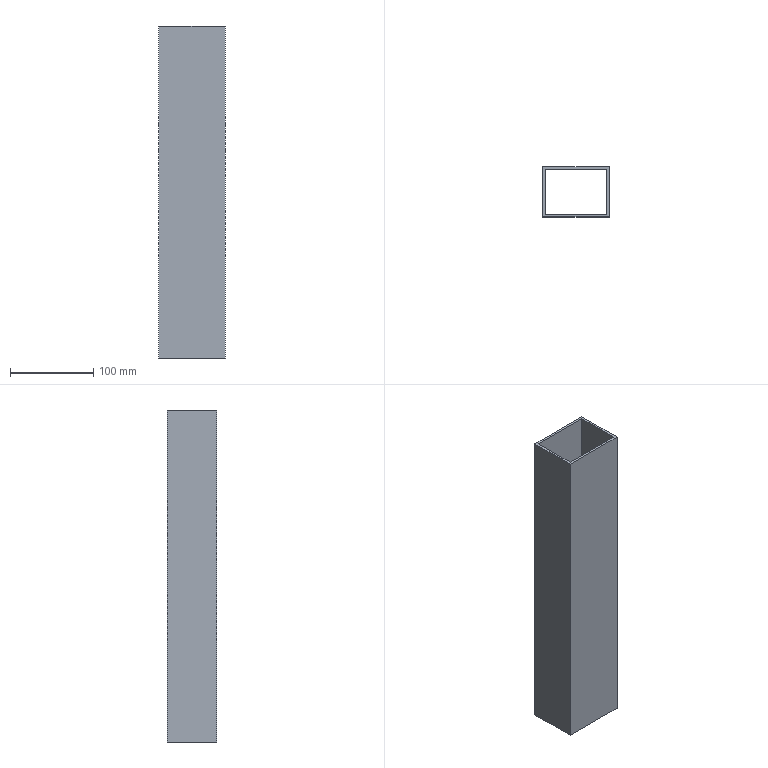Part | STEP file | Guide wheel mechanism revised.sldasm-Part-151 | 1 solid | 10 faces | box 80 x 60 x 400 mm | volume 321600 mm3 | plane 10
STEP:
#1=CARTESIAN_POINT('',(-360.,1970.,200.));
#2=VERTEX_POINT('',#1);
#3=CARTESIAN_POINT('',(-440.,1970.,200.));
#4=VERTEX_POINT('',#3);
#5=CARTESIAN_POINT('',(-440.,1970.,200.));
#6=DIRECTION('',(-1.,0.,0.));
#7=VECTOR('',#6,1000.);
#8=LINE('',#5,#7);
#9=EDGE_CURVE('',#2,#4,#8,.T.);
#10=ORIENTED_EDGE('',*,*,#9,.F.);
#11=CARTESIAN_POINT('',(-360.,1970.,-200.));
#12=VERTEX_POINT('',#11);
#13=CARTESIAN_POINT('',(-360.,1970.,300.));
#14=DIRECTION('',(0.,0.,-1.));
#15=VECTOR('',#14,1000.);
#16=LINE('',#13,#15);
#17=EDGE_CURVE('',#2,#12,#16,.T.);
#18=ORIENTED_EDGE('',*,*,#17,.T.);
#19=CARTESIAN_POINT('',(-440.,1970.,-200.));
#20=VERTEX_POINT('',#19);
#21=CARTESIAN_POINT('',(-440.,1970.,-200.));
#22=DIRECTION('',(-1.,0.,0.));
#23=VECTOR('',#22,1000.);
#24=LINE('',#21,#23);
#25=EDGE_CURVE('',#12,#20,#24,.T.);
#26=ORIENTED_EDGE('',*,*,#25,.T.);
#27=CARTESIAN_POINT('',(-440.,1970.,300.));
#28=DIRECTION('',(0.,0.,-1.));
#29=VECTOR('',#28,1000.);
#30=LINE('',#27,#29);
#31=EDGE_CURVE('',#4,#20,#30,.T.);
#32=ORIENTED_EDGE('',*,*,#31,.F.);
#33=EDGE_LOOP('',(#10,#18,#26,#32));
#34=FACE_OUTER_BOUND('',#33,.T.);
#35=CARTESIAN_POINT('',(-440.,1970.,300.));
#36=DIRECTION('',(0.,-1.,0.));
#37=DIRECTION('',(1.,0.,0.));
#38=AXIS2_PLACEMENT_3D('',#35,#36,#37);
#39=PLANE('',#38);
#40=ADVANCED_FACE('',(#34),#39,.F.);
#41=CARTESIAN_POINT('',(-360.,1910.,200.));
#42=VERTEX_POINT('',#41);
#43=CARTESIAN_POINT('',(-360.,1970.,200.));
#44=DIRECTION('',(0.,1.,0.));
#45=VECTOR('',#44,1000.);
#46=LINE('',#43,#45);
#47=EDGE_CURVE('',#42,#2,#46,.T.);
#48=ORIENTED_EDGE('',*,*,#47,.F.);
#49=CARTESIAN_POINT('',(-360.,1910.,-200.));
#50=VERTEX_POINT('',#49);
#51=CARTESIAN_POINT('',(-360.,1910.,300.));
#52=DIRECTION('',(0.,0.,-1.));
#53=VECTOR('',#52,1000.);
#54=LINE('',#51,#53);
#55=EDGE_CURVE('',#42,#50,#54,.T.);
#56=ORIENTED_EDGE('',*,*,#55,.T.);
#57=CARTESIAN_POINT('',(-360.,1970.,-200.));
#58=DIRECTION('',(0.,1.,0.));
#59=VECTOR('',#58,1000.);
#60=LINE('',#57,#59);
#61=EDGE_CURVE('',#50,#12,#60,.T.);
#62=ORIENTED_EDGE('',*,*,#61,.T.);
#63=ORIENTED_EDGE('',*,*,#17,.F.);
#64=EDGE_LOOP('',(#48,#56,#62,#63));
#65=FACE_OUTER_BOUND('',#64,.T.);
#66=CARTESIAN_POINT('',(-360.,1970.,300.));
#67=DIRECTION('',(-1.,0.,0.));
#68=DIRECTION('',(0.,0.,1.));
#69=AXIS2_PLACEMENT_3D('',#66,#67,#68);
#70=PLANE('',#69);
#71=ADVANCED_FACE('',(#65),#70,.F.);
#72=CARTESIAN_POINT('',(-440.,1910.,200.));
#73=VERTEX_POINT('',#72);
#74=CARTESIAN_POINT('',(-440.,1910.,200.));
#75=DIRECTION('',(1.,0.,0.));
#76=VECTOR('',#75,1000.);
#77=LINE('',#74,#76);
#78=EDGE_CURVE('',#73,#42,#77,.T.);
#79=ORIENTED_EDGE('',*,*,#78,.F.);
#80=CARTESIAN_POINT('',(-440.,1910.,-200.));
#81=VERTEX_POINT('',#80);
#82=CARTESIAN_POINT('',(-440.,1910.,300.));
#83=DIRECTION('',(0.,0.,-1.));
#84=VECTOR('',#83,1000.);
#85=LINE('',#82,#84);
#86=EDGE_CURVE('',#73,#81,#85,.T.);
#87=ORIENTED_EDGE('',*,*,#86,.T.);
#88=CARTESIAN_POINT('',(-440.,1910.,-200.));
#89=DIRECTION('',(1.,0.,0.));
#90=VECTOR('',#89,1000.);
#91=LINE('',#88,#90);
#92=EDGE_CURVE('',#81,#50,#91,.T.);
#93=ORIENTED_EDGE('',*,*,#92,.T.);
#94=ORIENTED_EDGE('',*,*,#55,.F.);
#95=EDGE_LOOP('',(#79,#87,#93,#94));
#96=FACE_OUTER_BOUND('',#95,.T.);
#97=CARTESIAN_POINT('',(-440.,1910.,300.));
#98=DIRECTION('',(0.,1.,0.));
#99=DIRECTION('',(0.,0.,1.));
#100=AXIS2_PLACEMENT_3D('',#97,#98,#99);
#101=PLANE('',#100);
#102=ADVANCED_FACE('',(#96),#101,.F.);
#103=CARTESIAN_POINT('',(-440.,1970.,200.));
#104=DIRECTION('',(0.,-1.,0.));
#105=VECTOR('',#104,1000.);
#106=LINE('',#103,#105);
#107=EDGE_CURVE('',#4,#73,#106,.T.);
#108=ORIENTED_EDGE('',*,*,#107,.F.);
#109=ORIENTED_EDGE('',*,*,#31,.T.);
#110=CARTESIAN_POINT('',(-440.,1970.,-200.));
#111=DIRECTION('',(0.,-1.,0.));
#112=VECTOR('',#111,1000.);
#113=LINE('',#110,#112);
#114=EDGE_CURVE('',#20,#81,#113,.T.);
#115=ORIENTED_EDGE('',*,*,#114,.T.);
#116=ORIENTED_EDGE('',*,*,#86,.F.);
#117=EDGE_LOOP('',(#108,#109,#115,#116));
#118=FACE_OUTER_BOUND('',#117,.T.);
#119=CARTESIAN_POINT('',(-440.,1970.,300.));
#120=DIRECTION('',(1.,0.,0.));
#121=DIRECTION('',(0.,0.,-1.));
#122=AXIS2_PLACEMENT_3D('',#119,#120,#121);
#123=PLANE('',#122);
#124=ADVANCED_FACE('',(#118),#123,.F.);
#125=ORIENTED_EDGE('',*,*,#114,.F.);
#126=ORIENTED_EDGE('',*,*,#25,.F.);
#127=ORIENTED_EDGE('',*,*,#61,.F.);
#128=ORIENTED_EDGE('',*,*,#92,.F.);
#129=EDGE_LOOP('',(#125,#126,#127,#128));
#130=FACE_OUTER_BOUND('',#129,.T.);
#131=CARTESIAN_POINT('',(-437.,1967.,-200.));
#132=VERTEX_POINT('',#131);
#133=CARTESIAN_POINT('',(-437.,1913.,-200.));
#134=VERTEX_POINT('',#133);
#135=CARTESIAN_POINT('',(-437.,1967.,-200.));
#136=DIRECTION('',(0.,-1.,0.));
#137=VECTOR('',#136,1000.);
#138=LINE('',#135,#137);
#139=EDGE_CURVE('',#132,#134,#138,.T.);
#140=ORIENTED_EDGE('',*,*,#139,.T.);
#141=CARTESIAN_POINT('',(-363.,1913.,-200.));
#142=VERTEX_POINT('',#141);
#143=CARTESIAN_POINT('',(-437.,1913.,-200.));
#144=DIRECTION('',(1.,0.,0.));
#145=VECTOR('',#144,1000.);
#146=LINE('',#143,#145);
#147=EDGE_CURVE('',#134,#142,#146,.T.);
#148=ORIENTED_EDGE('',*,*,#147,.T.);
#149=CARTESIAN_POINT('',(-363.,1967.,-200.));
#150=VERTEX_POINT('',#149);
#151=CARTESIAN_POINT('',(-363.,1967.,-200.));
#152=DIRECTION('',(0.,1.,0.));
#153=VECTOR('',#152,1000.);
#154=LINE('',#151,#153);
#155=EDGE_CURVE('',#142,#150,#154,.T.);
#156=ORIENTED_EDGE('',*,*,#155,.T.);
#157=CARTESIAN_POINT('',(-437.,1967.,-200.));
#158=DIRECTION('',(-1.,0.,0.));
#159=VECTOR('',#158,1000.);
#160=LINE('',#157,#159);
#161=EDGE_CURVE('',#150,#132,#160,.T.);
#162=ORIENTED_EDGE('',*,*,#161,.T.);
#163=EDGE_LOOP('',(#140,#148,#156,#162));
#164=FACE_BOUND('',#163,.T.);
#165=CARTESIAN_POINT('',(0.,0.,-200.));
#166=DIRECTION('',(0.,0.,1.));
#167=DIRECTION('',(1.,0.,0.));
#168=AXIS2_PLACEMENT_3D('',#165,#166,#167);
#169=PLANE('',#168);
#170=ADVANCED_FACE('',(#130,#164),#169,.F.);
#171=CARTESIAN_POINT('',(-363.,1967.,200.));
#172=VERTEX_POINT('',#171);
#173=CARTESIAN_POINT('',(-363.,1967.,300.));
#174=DIRECTION('',(0.,0.,-1.));
#175=VECTOR('',#174,1000.);
#176=LINE('',#173,#175);
#177=EDGE_CURVE('',#172,#150,#176,.T.);
#178=ORIENTED_EDGE('',*,*,#177,.F.);
#179=CARTESIAN_POINT('',(-437.,1967.,200.));
#180=VERTEX_POINT('',#179);
#181=CARTESIAN_POINT('',(-437.,1967.,200.));
#182=DIRECTION('',(-1.,0.,0.));
#183=VECTOR('',#182,1000.);
#184=LINE('',#181,#183);
#185=EDGE_CURVE('',#172,#180,#184,.T.);
#186=ORIENTED_EDGE('',*,*,#185,.T.);
#187=CARTESIAN_POINT('',(-437.,1967.,300.));
#188=DIRECTION('',(0.,0.,-1.));
#189=VECTOR('',#188,1000.);
#190=LINE('',#187,#189);
#191=EDGE_CURVE('',#180,#132,#190,.T.);
#192=ORIENTED_EDGE('',*,*,#191,.T.);
#193=ORIENTED_EDGE('',*,*,#161,.F.);
#194=EDGE_LOOP('',(#178,#186,#192,#193));
#195=FACE_OUTER_BOUND('',#194,.T.);
#196=CARTESIAN_POINT('',(-437.,1967.,300.));
#197=DIRECTION('',(0.,-1.,0.));
#198=DIRECTION('',(0.,0.,-1.));
#199=AXIS2_PLACEMENT_3D('',#196,#197,#198);
#200=PLANE('',#199);
#201=ADVANCED_FACE('',(#195),#200,.T.);
#202=CARTESIAN_POINT('',(-363.,1913.,200.));
#203=VERTEX_POINT('',#202);
#204=CARTESIAN_POINT('',(-363.,1913.,300.));
#205=DIRECTION('',(0.,0.,-1.));
#206=VECTOR('',#205,1000.);
#207=LINE('',#204,#206);
#208=EDGE_CURVE('',#203,#142,#207,.T.);
#209=ORIENTED_EDGE('',*,*,#208,.F.);
#210=CARTESIAN_POINT('',(-363.,1967.,200.));
#211=DIRECTION('',(0.,1.,0.));
#212=VECTOR('',#211,1000.);
#213=LINE('',#210,#212);
#214=EDGE_CURVE('',#203,#172,#213,.T.);
#215=ORIENTED_EDGE('',*,*,#214,.T.);
#216=ORIENTED_EDGE('',*,*,#177,.T.);
#217=ORIENTED_EDGE('',*,*,#155,.F.);
#218=EDGE_LOOP('',(#209,#215,#216,#217));
#219=FACE_OUTER_BOUND('',#218,.T.);
#220=CARTESIAN_POINT('',(-363.,1967.,300.));
#221=DIRECTION('',(-1.,0.,0.));
#222=DIRECTION('',(0.,0.,1.));
#223=AXIS2_PLACEMENT_3D('',#220,#221,#222);
#224=PLANE('',#223);
#225=ADVANCED_FACE('',(#219),#224,.T.);
#226=CARTESIAN_POINT('',(-437.,1913.,200.));
#227=VERTEX_POINT('',#226);
#228=CARTESIAN_POINT('',(-437.,1913.,300.));
#229=DIRECTION('',(0.,0.,-1.));
#230=VECTOR('',#229,1000.);
#231=LINE('',#228,#230);
#232=EDGE_CURVE('',#227,#134,#231,.T.);
#233=ORIENTED_EDGE('',*,*,#232,.F.);
#234=CARTESIAN_POINT('',(-437.,1913.,200.));
#235=DIRECTION('',(1.,0.,0.));
#236=VECTOR('',#235,1000.);
#237=LINE('',#234,#236);
#238=EDGE_CURVE('',#227,#203,#237,.T.);
#239=ORIENTED_EDGE('',*,*,#238,.T.);
#240=ORIENTED_EDGE('',*,*,#208,.T.);
#241=ORIENTED_EDGE('',*,*,#147,.F.);
#242=EDGE_LOOP('',(#233,#239,#240,#241));
#243=FACE_OUTER_BOUND('',#242,.T.);
#244=CARTESIAN_POINT('',(-437.,1913.,300.));
#245=DIRECTION('',(0.,1.,0.));
#246=DIRECTION('',(0.,0.,1.));
#247=AXIS2_PLACEMENT_3D('',#244,#245,#246);
#248=PLANE('',#247);
#249=ADVANCED_FACE('',(#243),#248,.T.);
#250=ORIENTED_EDGE('',*,*,#191,.F.);
#251=CARTESIAN_POINT('',(-437.,1967.,200.));
#252=DIRECTION('',(0.,-1.,0.));
#253=VECTOR('',#252,1000.);
#254=LINE('',#251,#253);
#255=EDGE_CURVE('',#180,#227,#254,.T.);
#256=ORIENTED_EDGE('',*,*,#255,.T.);
#257=ORIENTED_EDGE('',*,*,#232,.T.);
#258=ORIENTED_EDGE('',*,*,#139,.F.);
#259=EDGE_LOOP('',(#250,#256,#257,#258));
#260=FACE_OUTER_BOUND('',#259,.T.);
#261=CARTESIAN_POINT('',(-437.,1967.,300.));
#262=DIRECTION('',(1.,0.,0.));
#263=DIRECTION('',(0.,1.,0.));
#264=AXIS2_PLACEMENT_3D('',#261,#262,#263);
#265=PLANE('',#264);
#266=ADVANCED_FACE('',(#260),#265,.T.);
#267=ORIENTED_EDGE('',*,*,#255,.F.);
#268=ORIENTED_EDGE('',*,*,#185,.F.);
#269=ORIENTED_EDGE('',*,*,#214,.F.);
#270=ORIENTED_EDGE('',*,*,#238,.F.);
#271=EDGE_LOOP('',(#267,#268,#269,#270));
#272=FACE_BOUND('',#271,.T.);
#273=ORIENTED_EDGE('',*,*,#9,.T.);
#274=ORIENTED_EDGE('',*,*,#107,.T.);
#275=ORIENTED_EDGE('',*,*,#78,.T.);
#276=ORIENTED_EDGE('',*,*,#47,.T.);
#277=EDGE_LOOP('',(#273,#274,#275,#276));
#278=FACE_OUTER_BOUND('',#277,.T.);
#279=CARTESIAN_POINT('',(-360.,1970.,200.));
#280=DIRECTION('',(0.,0.,1.));
#281=DIRECTION('',(1.,0.,0.));
#282=AXIS2_PLACEMENT_3D('',#279,#280,#281);
#283=PLANE('',#282);
#284=ADVANCED_FACE('',(#272,#278),#283,.T.);
#285=CLOSED_SHELL('',(#40,#71,#102,#124,#170,#201,#225,#249,#266,#284));
#286=MANIFOLD_SOLID_BREP('',#285);
#287=CARTESIAN_POINT('',(0.,0.,0.));
#288=DIRECTION('',(0.,0.,1.));
#289=DIRECTION('',(1.,0.,0.));
#290=AXIS2_PLACEMENT_3D('',#287,#288,#289);
#291=(LENGTH_UNIT()NAMED_UNIT(*)SI_UNIT(.MILLI.,.METRE.));
#292=UNCERTAINTY_MEASURE_WITH_UNIT(LENGTH_MEASURE(0.00001),#291,'','');
#293=(NAMED_UNIT(*)PLANE_ANGLE_UNIT()SI_UNIT($,.RADIAN.));
#294=(NAMED_UNIT(*)SI_UNIT($,.STERADIAN.)SOLID_ANGLE_UNIT());
#295=(GEOMETRIC_REPRESENTATION_CONTEXT(3)GLOBAL_UNCERTAINTY_ASSIGNED_CONTEXT((#292))GLOBAL_UNIT_ASSIGNED_CONTEXT((#291,#293,#294))REPRESENTATION_CONTEXT('',''));
#296=ADVANCED_BREP_SHAPE_REPRESENTATION('',(#286,#290),#295);